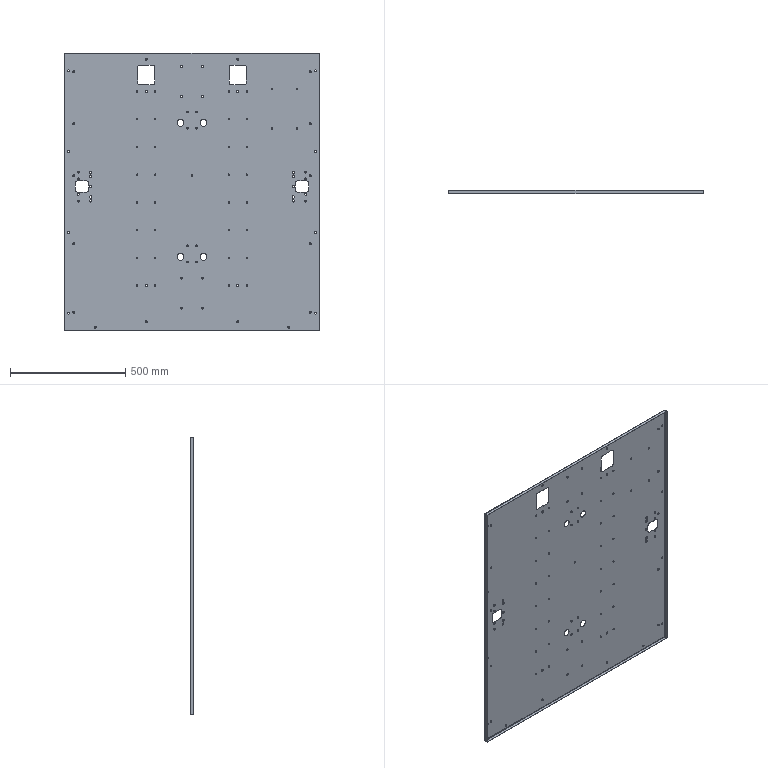Part | SolidWorks | features HoleWzd 7, Cut 2, EdgeFlange 1, FlatPattern 1, LPattern 1, MirrorPattern 1, SMBaseFlange 1, SheetMetal 1 | 1 solid | 276 faces | box 1104 x 15 x 1204 mm | volume 1365572 mm3 | cylinder 230 | plane 38 | spline 8 | commonest cylinder face diameters 8.5 x66 6 x64 8 x32 10 x16 11 x12 6.5 x8